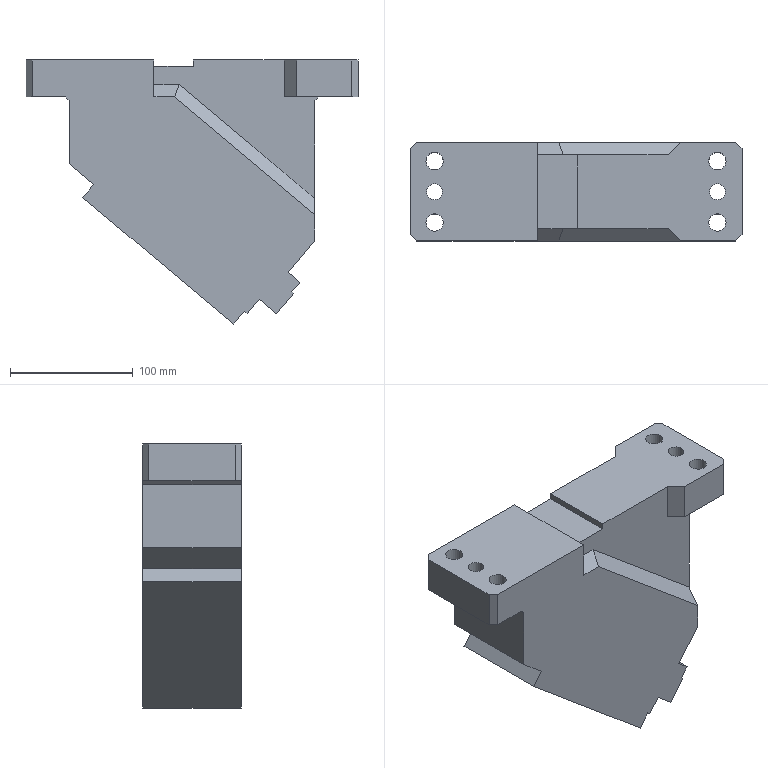Part | NX | features solid 2 | 1 solid | 55 faces | box 270 x 80 x 214.702 mm | volume 2651547 mm3 | plane 45 | cylinder 10 | commonest cylinder face diameters 14 x4 20 x4 13 x2